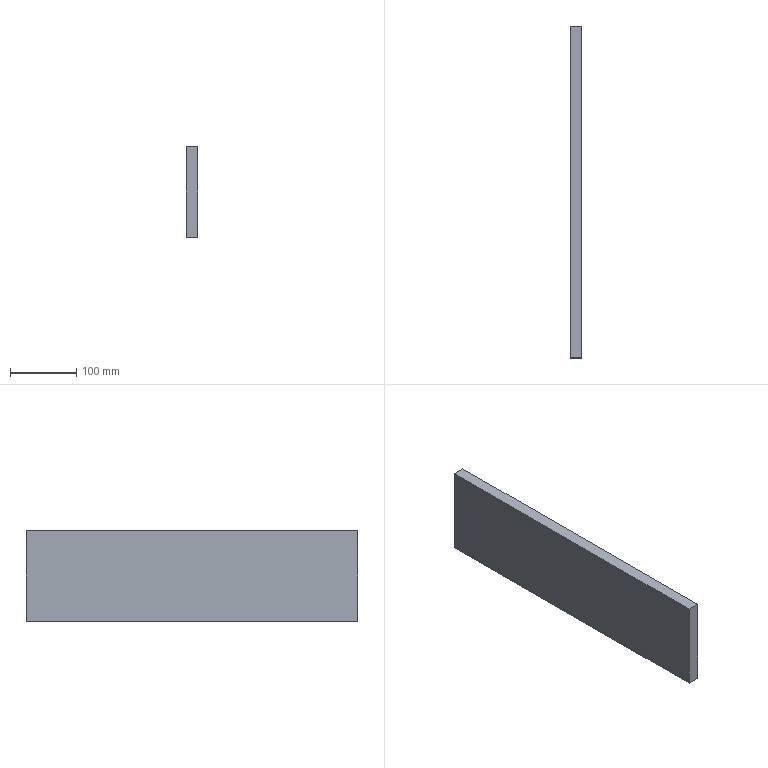Part | STEP file | Middle_part | 1 solid | 6 faces | box 18 x 502 x 137 mm | volume 1237932 mm3 | plane 6
STEP:
#1=CARTESIAN_POINT('',(0.,0.,0.));
#2=DIRECTION('',(0.,0.,1.));
#3=DIRECTION('',(1.,0.,0.));
#4=AXIS2_PLACEMENT_3D('',#1,#2,#3);
#5=CARTESIAN_POINT('',(-9.,251.,68.5));
#6=VERTEX_POINT('',#5);
#7=CARTESIAN_POINT('',(-9.,-251.,68.5));
#8=VERTEX_POINT('',#7);
#9=CARTESIAN_POINT('',(-9.,251.,68.5));
#10=DIRECTION('',(0.,-1.,0.));
#11=VECTOR('',#10,1.);
#12=LINE('',#9,#11);
#13=CARTESIAN_POINT('',(-9.,251.,68.5));
#14=DIRECTION('',(1.,0.,0.));
#15=DIRECTION('',(0.,0.,-1.));
#16=AXIS2_PLACEMENT_3D('',#13,#14,#15);
#17=PLANE('',#16);
#18=CARTESIAN_POINT('',(0.,0.));
#19=DIRECTION('',(0.,-1.));
#20=VECTOR('',#19,1.);
#21=LINE('',#18,#20);
#22=(GEOMETRIC_REPRESENTATION_CONTEXT(2)PARAMETRIC_REPRESENTATION_CONTEXT()REPRESENTATION_CONTEXT('',''));
#23=DEFINITIONAL_REPRESENTATION('',(#21),#22);
#24=PCURVE('',#17,#23);
#25=CARTESIAN_POINT('',(9.,251.,68.5));
#26=DIRECTION('',(0.,0.,-1.));
#27=DIRECTION('',(-1.,0.,0.));
#28=AXIS2_PLACEMENT_3D('',#25,#26,#27);
#29=PLANE('',#28);
#30=CARTESIAN_POINT('',(18.,0.));
#31=DIRECTION('',(0.,-1.));
#32=VECTOR('',#31,1.);
#33=LINE('',#30,#32);
#34=(GEOMETRIC_REPRESENTATION_CONTEXT(2)PARAMETRIC_REPRESENTATION_CONTEXT()REPRESENTATION_CONTEXT('',''));
#35=DEFINITIONAL_REPRESENTATION('',(#33),#34);
#36=PCURVE('',#29,#35);
#37=SURFACE_CURVE('',#12,(#24,#36),.PCURVE_S1.);
#38=EDGE_CURVE('',#6,#8,#37,.T.);
#39=ORIENTED_EDGE('',*,*,#38,.T.);
#40=CARTESIAN_POINT('',(-9.,-251.,-68.5));
#41=VERTEX_POINT('',#40);
#42=CARTESIAN_POINT('',(-9.,-251.,68.5));
#43=DIRECTION('',(0.,0.,-1.));
#44=VECTOR('',#43,1.);
#45=LINE('',#42,#44);
#46=CARTESIAN_POINT('',(0.,-502.));
#47=DIRECTION('',(1.,0.));
#48=VECTOR('',#47,1.);
#49=LINE('',#46,#48);
#50=(GEOMETRIC_REPRESENTATION_CONTEXT(2)PARAMETRIC_REPRESENTATION_CONTEXT()REPRESENTATION_CONTEXT('',''));
#51=DEFINITIONAL_REPRESENTATION('',(#49),#50);
#52=PCURVE('',#17,#51);
#53=CARTESIAN_POINT('',(0.,-251.,0.));
#54=DIRECTION('',(0.,1.,0.));
#55=DIRECTION('',(0.,0.,1.));
#56=AXIS2_PLACEMENT_3D('',#53,#54,#55);
#57=PLANE('',#56);
#58=CARTESIAN_POINT('',(68.5,-9.));
#59=DIRECTION('',(-1.,0.));
#60=VECTOR('',#59,1.);
#61=LINE('',#58,#60);
#62=(GEOMETRIC_REPRESENTATION_CONTEXT(2)PARAMETRIC_REPRESENTATION_CONTEXT()REPRESENTATION_CONTEXT('',''));
#63=DEFINITIONAL_REPRESENTATION('',(#61),#62);
#64=PCURVE('',#57,#63);
#65=SURFACE_CURVE('',#45,(#52,#64),.PCURVE_S1.);
#66=EDGE_CURVE('',#8,#41,#65,.T.);
#67=ORIENTED_EDGE('',*,*,#66,.T.);
#68=CARTESIAN_POINT('',(-9.,251.,-68.5));
#69=VERTEX_POINT('',#68);
#70=CARTESIAN_POINT('',(-9.,251.,-68.5));
#71=DIRECTION('',(0.,-1.,0.));
#72=VECTOR('',#71,1.);
#73=LINE('',#70,#72);
#74=CARTESIAN_POINT('',(137.,0.));
#75=DIRECTION('',(0.,-1.));
#76=VECTOR('',#75,1.);
#77=LINE('',#74,#76);
#78=(GEOMETRIC_REPRESENTATION_CONTEXT(2)PARAMETRIC_REPRESENTATION_CONTEXT()REPRESENTATION_CONTEXT('',''));
#79=DEFINITIONAL_REPRESENTATION('',(#77),#78);
#80=PCURVE('',#17,#79);
#81=CARTESIAN_POINT('',(-9.,251.,-68.5));
#82=DIRECTION('',(0.,0.,1.));
#83=DIRECTION('',(1.,0.,0.));
#84=AXIS2_PLACEMENT_3D('',#81,#82,#83);
#85=PLANE('',#84);
#86=CARTESIAN_POINT('',(0.,0.));
#87=DIRECTION('',(0.,-1.));
#88=VECTOR('',#87,1.);
#89=LINE('',#86,#88);
#90=(GEOMETRIC_REPRESENTATION_CONTEXT(2)PARAMETRIC_REPRESENTATION_CONTEXT()REPRESENTATION_CONTEXT('',''));
#91=DEFINITIONAL_REPRESENTATION('',(#89),#90);
#92=PCURVE('',#85,#91);
#93=SURFACE_CURVE('',#73,(#80,#92),.PCURVE_S1.);
#94=EDGE_CURVE('',#69,#41,#93,.T.);
#95=ORIENTED_EDGE('',*,*,#94,.F.);
#96=CARTESIAN_POINT('',(-9.,251.,68.5));
#97=DIRECTION('',(0.,0.,-1.));
#98=VECTOR('',#97,1.);
#99=LINE('',#96,#98);
#100=CARTESIAN_POINT('',(0.,0.));
#101=DIRECTION('',(1.,0.));
#102=VECTOR('',#101,1.);
#103=LINE('',#100,#102);
#104=(GEOMETRIC_REPRESENTATION_CONTEXT(2)PARAMETRIC_REPRESENTATION_CONTEXT()REPRESENTATION_CONTEXT('',''));
#105=DEFINITIONAL_REPRESENTATION('',(#103),#104);
#106=PCURVE('',#17,#105);
#107=CARTESIAN_POINT('',(0.,251.,0.));
#108=DIRECTION('',(0.,1.,0.));
#109=DIRECTION('',(0.,0.,1.));
#110=AXIS2_PLACEMENT_3D('',#107,#108,#109);
#111=PLANE('',#110);
#112=CARTESIAN_POINT('',(68.5,-9.));
#113=DIRECTION('',(-1.,0.));
#114=VECTOR('',#113,1.);
#115=LINE('',#112,#114);
#116=(GEOMETRIC_REPRESENTATION_CONTEXT(2)PARAMETRIC_REPRESENTATION_CONTEXT()REPRESENTATION_CONTEXT('',''));
#117=DEFINITIONAL_REPRESENTATION('',(#115),#116);
#118=PCURVE('',#111,#117);
#119=SURFACE_CURVE('',#99,(#106,#118),.PCURVE_S1.);
#120=EDGE_CURVE('',#6,#69,#119,.T.);
#121=ORIENTED_EDGE('',*,*,#120,.F.);
#122=EDGE_LOOP('',(#39,#67,#95,#121));
#123=FACE_BOUND('',#122,.F.);
#124=ADVANCED_FACE('',(#123),#17,.F.);
#125=ORIENTED_EDGE('',*,*,#94,.T.);
#126=CARTESIAN_POINT('',(9.,-251.,-68.5));
#127=VERTEX_POINT('',#126);
#128=CARTESIAN_POINT('',(-9.,-251.,-68.5));
#129=DIRECTION('',(1.,0.,0.));
#130=VECTOR('',#129,1.);
#131=LINE('',#128,#130);
#132=CARTESIAN_POINT('',(0.,-502.));
#133=DIRECTION('',(1.,0.));
#134=VECTOR('',#133,1.);
#135=LINE('',#132,#134);
#136=(GEOMETRIC_REPRESENTATION_CONTEXT(2)PARAMETRIC_REPRESENTATION_CONTEXT()REPRESENTATION_CONTEXT('',''));
#137=DEFINITIONAL_REPRESENTATION('',(#135),#136);
#138=PCURVE('',#85,#137);
#139=CARTESIAN_POINT('',(-68.5,-9.));
#140=DIRECTION('',(0.,1.));
#141=VECTOR('',#140,1.);
#142=LINE('',#139,#141);
#143=(GEOMETRIC_REPRESENTATION_CONTEXT(2)PARAMETRIC_REPRESENTATION_CONTEXT()REPRESENTATION_CONTEXT('',''));
#144=DEFINITIONAL_REPRESENTATION('',(#142),#143);
#145=PCURVE('',#57,#144);
#146=SURFACE_CURVE('',#131,(#138,#145),.PCURVE_S1.);
#147=EDGE_CURVE('',#41,#127,#146,.T.);
#148=ORIENTED_EDGE('',*,*,#147,.T.);
#149=CARTESIAN_POINT('',(9.,251.,-68.5));
#150=VERTEX_POINT('',#149);
#151=CARTESIAN_POINT('',(9.,251.,-68.5));
#152=DIRECTION('',(0.,-1.,0.));
#153=VECTOR('',#152,1.);
#154=LINE('',#151,#153);
#155=CARTESIAN_POINT('',(18.,0.));
#156=DIRECTION('',(0.,-1.));
#157=VECTOR('',#156,1.);
#158=LINE('',#155,#157);
#159=(GEOMETRIC_REPRESENTATION_CONTEXT(2)PARAMETRIC_REPRESENTATION_CONTEXT()REPRESENTATION_CONTEXT('',''));
#160=DEFINITIONAL_REPRESENTATION('',(#158),#159);
#161=PCURVE('',#85,#160);
#162=CARTESIAN_POINT('',(9.,251.,-68.5));
#163=DIRECTION('',(-1.,0.,0.));
#164=DIRECTION('',(0.,0.,1.));
#165=AXIS2_PLACEMENT_3D('',#162,#163,#164);
#166=PLANE('',#165);
#167=CARTESIAN_POINT('',(0.,0.));
#168=DIRECTION('',(0.,-1.));
#169=VECTOR('',#168,1.);
#170=LINE('',#167,#169);
#171=(GEOMETRIC_REPRESENTATION_CONTEXT(2)PARAMETRIC_REPRESENTATION_CONTEXT()REPRESENTATION_CONTEXT('',''));
#172=DEFINITIONAL_REPRESENTATION('',(#170),#171);
#173=PCURVE('',#166,#172);
#174=SURFACE_CURVE('',#154,(#161,#173),.PCURVE_S1.);
#175=EDGE_CURVE('',#150,#127,#174,.T.);
#176=ORIENTED_EDGE('',*,*,#175,.F.);
#177=CARTESIAN_POINT('',(-9.,251.,-68.5));
#178=DIRECTION('',(1.,0.,0.));
#179=VECTOR('',#178,1.);
#180=LINE('',#177,#179);
#181=CARTESIAN_POINT('',(0.,0.));
#182=DIRECTION('',(1.,0.));
#183=VECTOR('',#182,1.);
#184=LINE('',#181,#183);
#185=(GEOMETRIC_REPRESENTATION_CONTEXT(2)PARAMETRIC_REPRESENTATION_CONTEXT()REPRESENTATION_CONTEXT('',''));
#186=DEFINITIONAL_REPRESENTATION('',(#184),#185);
#187=PCURVE('',#85,#186);
#188=CARTESIAN_POINT('',(-68.5,-9.));
#189=DIRECTION('',(0.,1.));
#190=VECTOR('',#189,1.);
#191=LINE('',#188,#190);
#192=(GEOMETRIC_REPRESENTATION_CONTEXT(2)PARAMETRIC_REPRESENTATION_CONTEXT()REPRESENTATION_CONTEXT('',''));
#193=DEFINITIONAL_REPRESENTATION('',(#191),#192);
#194=PCURVE('',#111,#193);
#195=SURFACE_CURVE('',#180,(#187,#194),.PCURVE_S1.);
#196=EDGE_CURVE('',#69,#150,#195,.T.);
#197=ORIENTED_EDGE('',*,*,#196,.F.);
#198=EDGE_LOOP('',(#125,#148,#176,#197));
#199=FACE_BOUND('',#198,.F.);
#200=ADVANCED_FACE('',(#199),#85,.F.);
#201=ORIENTED_EDGE('',*,*,#175,.T.);
#202=CARTESIAN_POINT('',(9.,-251.,68.5));
#203=VERTEX_POINT('',#202);
#204=CARTESIAN_POINT('',(9.,-251.,-68.5));
#205=DIRECTION('',(0.,0.,1.));
#206=VECTOR('',#205,1.);
#207=LINE('',#204,#206);
#208=CARTESIAN_POINT('',(0.,-502.));
#209=DIRECTION('',(1.,0.));
#210=VECTOR('',#209,1.);
#211=LINE('',#208,#210);
#212=(GEOMETRIC_REPRESENTATION_CONTEXT(2)PARAMETRIC_REPRESENTATION_CONTEXT()REPRESENTATION_CONTEXT('',''));
#213=DEFINITIONAL_REPRESENTATION('',(#211),#212);
#214=PCURVE('',#166,#213);
#215=CARTESIAN_POINT('',(-68.5,9.));
#216=DIRECTION('',(1.,0.));
#217=VECTOR('',#216,1.);
#218=LINE('',#215,#217);
#219=(GEOMETRIC_REPRESENTATION_CONTEXT(2)PARAMETRIC_REPRESENTATION_CONTEXT()REPRESENTATION_CONTEXT('',''));
#220=DEFINITIONAL_REPRESENTATION('',(#218),#219);
#221=PCURVE('',#57,#220);
#222=SURFACE_CURVE('',#207,(#214,#221),.PCURVE_S1.);
#223=EDGE_CURVE('',#127,#203,#222,.T.);
#224=ORIENTED_EDGE('',*,*,#223,.T.);
#225=CARTESIAN_POINT('',(9.,251.,68.5));
#226=VERTEX_POINT('',#225);
#227=CARTESIAN_POINT('',(9.,251.,68.5));
#228=DIRECTION('',(0.,-1.,0.));
#229=VECTOR('',#228,1.);
#230=LINE('',#227,#229);
#231=CARTESIAN_POINT('',(137.,0.));
#232=DIRECTION('',(0.,-1.));
#233=VECTOR('',#232,1.);
#234=LINE('',#231,#233);
#235=(GEOMETRIC_REPRESENTATION_CONTEXT(2)PARAMETRIC_REPRESENTATION_CONTEXT()REPRESENTATION_CONTEXT('',''));
#236=DEFINITIONAL_REPRESENTATION('',(#234),#235);
#237=PCURVE('',#166,#236);
#238=CARTESIAN_POINT('',(0.,0.));
#239=DIRECTION('',(0.,-1.));
#240=VECTOR('',#239,1.);
#241=LINE('',#238,#240);
#242=(GEOMETRIC_REPRESENTATION_CONTEXT(2)PARAMETRIC_REPRESENTATION_CONTEXT()REPRESENTATION_CONTEXT('',''));
#243=DEFINITIONAL_REPRESENTATION('',(#241),#242);
#244=PCURVE('',#29,#243);
#245=SURFACE_CURVE('',#230,(#237,#244),.PCURVE_S1.);
#246=EDGE_CURVE('',#226,#203,#245,.T.);
#247=ORIENTED_EDGE('',*,*,#246,.F.);
#248=CARTESIAN_POINT('',(9.,251.,-68.5));
#249=DIRECTION('',(0.,0.,1.));
#250=VECTOR('',#249,1.);
#251=LINE('',#248,#250);
#252=CARTESIAN_POINT('',(0.,0.));
#253=DIRECTION('',(1.,0.));
#254=VECTOR('',#253,1.);
#255=LINE('',#252,#254);
#256=(GEOMETRIC_REPRESENTATION_CONTEXT(2)PARAMETRIC_REPRESENTATION_CONTEXT()REPRESENTATION_CONTEXT('',''));
#257=DEFINITIONAL_REPRESENTATION('',(#255),#256);
#258=PCURVE('',#166,#257);
#259=CARTESIAN_POINT('',(-68.5,9.));
#260=DIRECTION('',(1.,0.));
#261=VECTOR('',#260,1.);
#262=LINE('',#259,#261);
#263=(GEOMETRIC_REPRESENTATION_CONTEXT(2)PARAMETRIC_REPRESENTATION_CONTEXT()REPRESENTATION_CONTEXT('',''));
#264=DEFINITIONAL_REPRESENTATION('',(#262),#263);
#265=PCURVE('',#111,#264);
#266=SURFACE_CURVE('',#251,(#258,#265),.PCURVE_S1.);
#267=EDGE_CURVE('',#150,#226,#266,.T.);
#268=ORIENTED_EDGE('',*,*,#267,.F.);
#269=EDGE_LOOP('',(#201,#224,#247,#268));
#270=FACE_BOUND('',#269,.F.);
#271=ADVANCED_FACE('',(#270),#166,.F.);
#272=ORIENTED_EDGE('',*,*,#246,.T.);
#273=CARTESIAN_POINT('',(9.,-251.,68.5));
#274=DIRECTION('',(-1.,0.,0.));
#275=VECTOR('',#274,1.);
#276=LINE('',#273,#275);
#277=CARTESIAN_POINT('',(0.,-502.));
#278=DIRECTION('',(1.,0.));
#279=VECTOR('',#278,1.);
#280=LINE('',#277,#279);
#281=(GEOMETRIC_REPRESENTATION_CONTEXT(2)PARAMETRIC_REPRESENTATION_CONTEXT()REPRESENTATION_CONTEXT('',''));
#282=DEFINITIONAL_REPRESENTATION('',(#280),#281);
#283=PCURVE('',#29,#282);
#284=CARTESIAN_POINT('',(68.5,9.));
#285=DIRECTION('',(0.,-1.));
#286=VECTOR('',#285,1.);
#287=LINE('',#284,#286);
#288=(GEOMETRIC_REPRESENTATION_CONTEXT(2)PARAMETRIC_REPRESENTATION_CONTEXT()REPRESENTATION_CONTEXT('',''));
#289=DEFINITIONAL_REPRESENTATION('',(#287),#288);
#290=PCURVE('',#57,#289);
#291=SURFACE_CURVE('',#276,(#283,#290),.PCURVE_S1.);
#292=EDGE_CURVE('',#203,#8,#291,.T.);
#293=ORIENTED_EDGE('',*,*,#292,.T.);
#294=ORIENTED_EDGE('',*,*,#38,.F.);
#295=CARTESIAN_POINT('',(9.,251.,68.5));
#296=DIRECTION('',(-1.,0.,0.));
#297=VECTOR('',#296,1.);
#298=LINE('',#295,#297);
#299=CARTESIAN_POINT('',(0.,0.));
#300=DIRECTION('',(1.,0.));
#301=VECTOR('',#300,1.);
#302=LINE('',#299,#301);
#303=(GEOMETRIC_REPRESENTATION_CONTEXT(2)PARAMETRIC_REPRESENTATION_CONTEXT()REPRESENTATION_CONTEXT('',''));
#304=DEFINITIONAL_REPRESENTATION('',(#302),#303);
#305=PCURVE('',#29,#304);
#306=CARTESIAN_POINT('',(68.5,9.));
#307=DIRECTION('',(0.,-1.));
#308=VECTOR('',#307,1.);
#309=LINE('',#306,#308);
#310=(GEOMETRIC_REPRESENTATION_CONTEXT(2)PARAMETRIC_REPRESENTATION_CONTEXT()REPRESENTATION_CONTEXT('',''));
#311=DEFINITIONAL_REPRESENTATION('',(#309),#310);
#312=PCURVE('',#111,#311);
#313=SURFACE_CURVE('',#298,(#305,#312),.PCURVE_S1.);
#314=EDGE_CURVE('',#226,#6,#313,.T.);
#315=ORIENTED_EDGE('',*,*,#314,.F.);
#316=EDGE_LOOP('',(#272,#293,#294,#315));
#317=FACE_BOUND('',#316,.F.);
#318=ADVANCED_FACE('',(#317),#29,.F.);
#319=ORIENTED_EDGE('',*,*,#120,.T.);
#320=ORIENTED_EDGE('',*,*,#196,.T.);
#321=ORIENTED_EDGE('',*,*,#267,.T.);
#322=ORIENTED_EDGE('',*,*,#314,.T.);
#323=EDGE_LOOP('',(#319,#320,#321,#322));
#324=FACE_BOUND('',#323,.F.);
#325=ADVANCED_FACE('',(#324),#111,.T.);
#326=ORIENTED_EDGE('',*,*,#66,.T.);
#327=ORIENTED_EDGE('',*,*,#147,.T.);
#328=ORIENTED_EDGE('',*,*,#223,.T.);
#329=ORIENTED_EDGE('',*,*,#292,.T.);
#330=EDGE_LOOP('',(#326,#327,#328,#329));
#331=FACE_BOUND('',#330,.T.);
#332=ADVANCED_FACE('',(#331),#57,.F.);
#333=CLOSED_SHELL('',(#124,#200,#271,#318,#325,#332));
#334=MANIFOLD_SOLID_BREP('',#333);
#335=(LENGTH_UNIT()NAMED_UNIT(*)SI_UNIT(.MILLI.,.METRE.));
#336=UNCERTAINTY_MEASURE_WITH_UNIT(LENGTH_MEASURE(0.0000001),#335,'','');
#337=(NAMED_UNIT(*)PLANE_ANGLE_UNIT()SI_UNIT($,.RADIAN.));
#338=(NAMED_UNIT(*)SI_UNIT($,.STERADIAN.)SOLID_ANGLE_UNIT());
#339=(GEOMETRIC_REPRESENTATION_CONTEXT(3)GLOBAL_UNCERTAINTY_ASSIGNED_CONTEXT((#336))GLOBAL_UNIT_ASSIGNED_CONTEXT((#335,#337,#338))REPRESENTATION_CONTEXT('',''));
#340=ADVANCED_BREP_SHAPE_REPRESENTATION('',(#4,#334),#339);